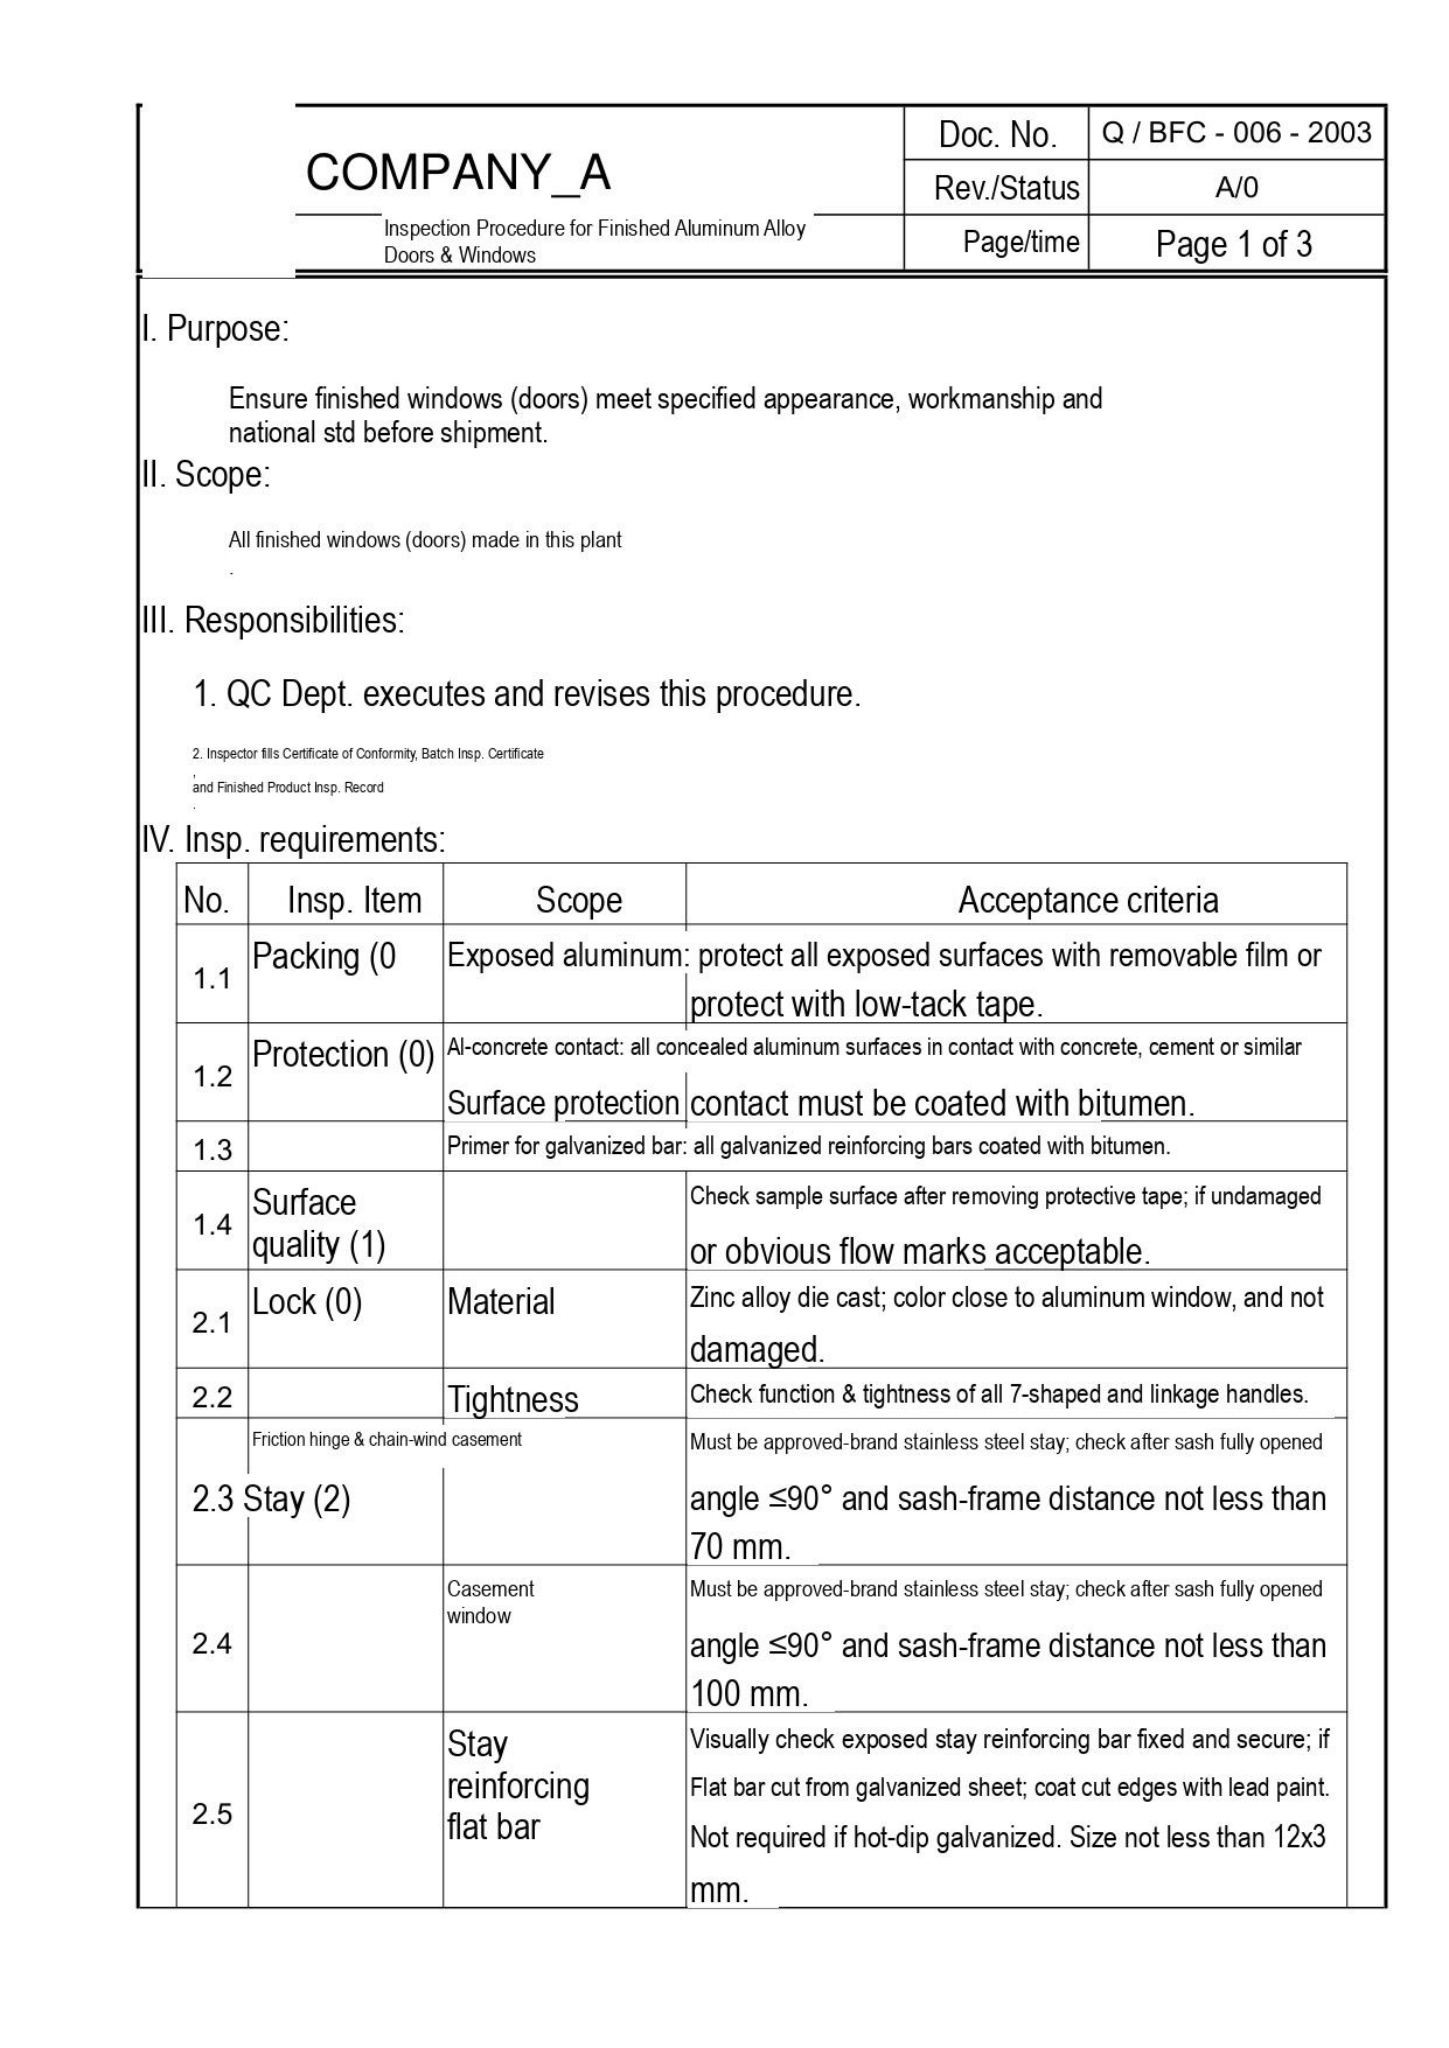COMPANY_A

Inspection Procedure for Finished Aluminum Alloy Doors & Windows

| Doc. No. | Q / BFC - 006 - 2003 |
|---|---|
| Rev./Status | A/0 |
| Page/time | Page 1 of 3 |

I. Purpose:

Ensure finished windows (doors) meet specified appearance, workmanship and national std before shipment.

II. Scope:

All finished windows (doors) made in this plant

III. Responsibilities:

1. QC Dept. executes and revises this procedure.

2. Inspector fills Certificate of Conformity, Batch Insp. Certificate and Finished Product Insp. Record

IV. Insp. requirements:

| No. | Insp. Item | Scope | Acceptance criteria |
|---|---|---|---|
| 1.1 | Packing (0 | Exposed aluminum: | protect all exposed surfaces with removable film or protect with low-tack tape. |
| 1.2 | Protection (0) | Al-concrete contact: Surface protection | all concealed aluminum surfaces in contact with concrete, cement or similar contact must be coated with bitumen. |
| 1.3 | | Primer for galvanized bar: | all galvanized reinforcing bars coated with bitumen. |
| 1.4 | Surface quality (1) | | Check sample surface after removing protective tape; if undamaged or obvious flow marks acceptable. |
| 2.1 | Lock (0) | Material | Zinc alloy die cast; color close to aluminum window, and not damaged. |
| 2.2 | | Tightness | Check function & tightness of all 7-shaped and linkage handles. |
| 2.3 | Stay (2) | Friction hinge & chain-wind casement | Must be approved-brand stainless steel stay; check after sash fully opened angle ≤90° and sash-frame distance not less than 70 mm. |
| 2.4 | | Casement window | Must be approved-brand stainless steel stay; check after sash fully opened angle ≤90° and sash-frame distance not less than 100 mm. |
| 2.5 | | Stay reinforcing flat bar | Visually check exposed stay reinforcing bar fixed and secure; if Flat bar cut from galvanized sheet; coat cut edges with lead paint. Not required if hot-dip galvanized. Size not less than 12x3 mm. |
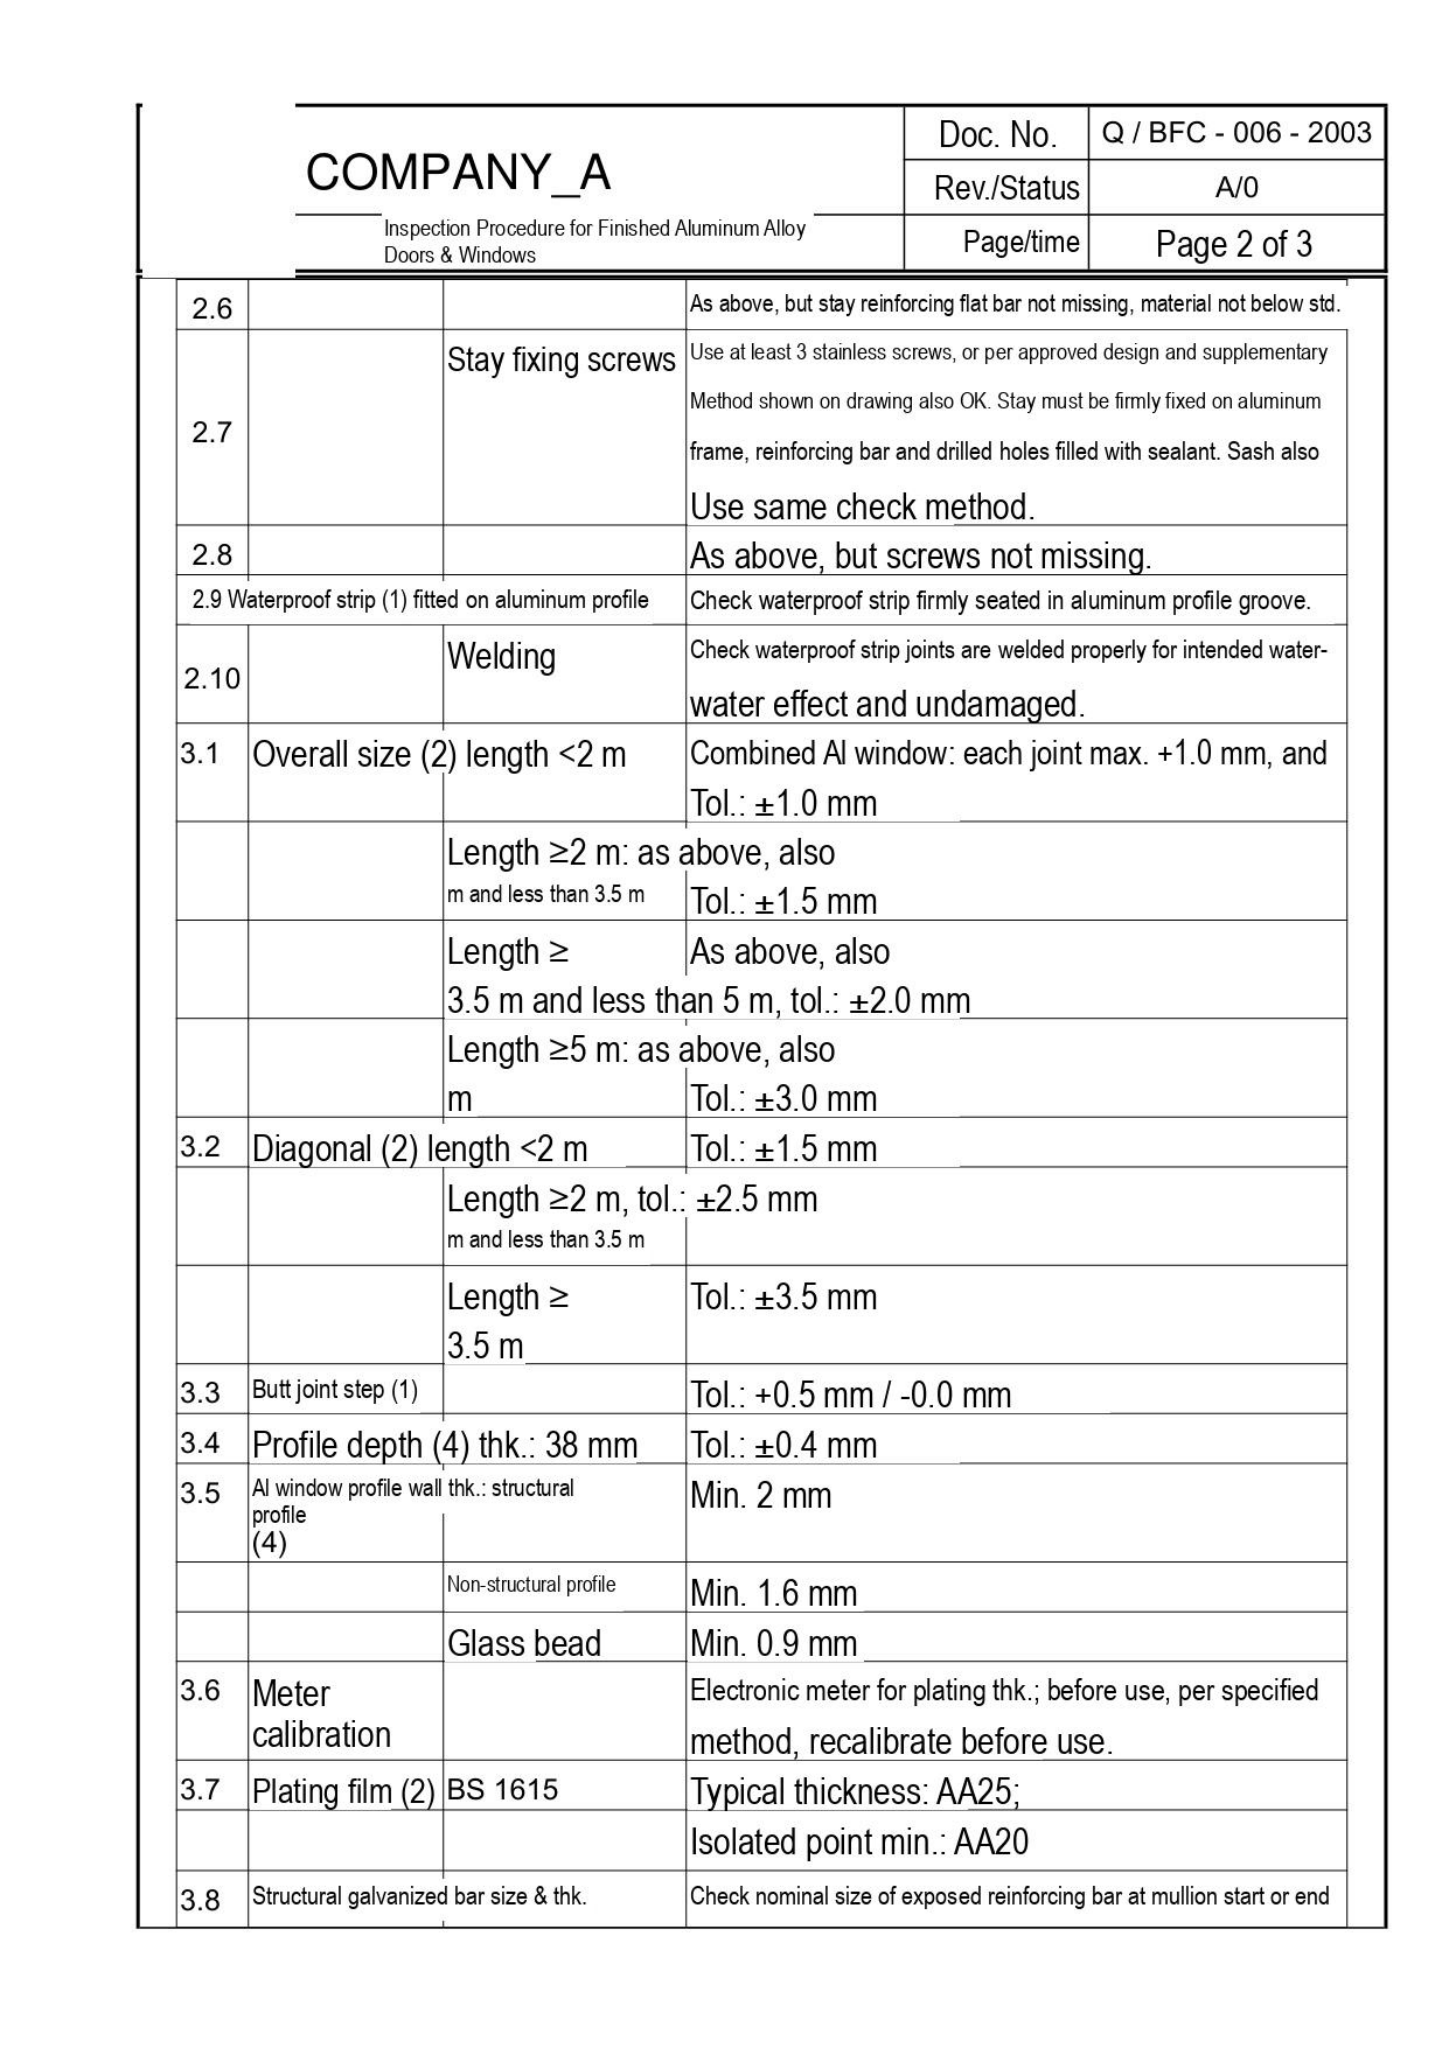| COMPANY_A<br>Inspection Procedure for Finished Aluminum Alloy Doors & Windows | Doc. No. | Q / BFC - 006 - 2003 |
|---|---|---|
| | Rev./Status | A/0 |
| | Page/time | Page 2 of 3 |

| | | | |
|---|---|---|---|
| 2.6 | | | As above, but stay reinforcing flat bar not missing, material not below std. |
| 2.7 | | Stay fixing screws | Use at least 3 stainless screws, or per approved design and supplementary Method shown on drawing also OK. Stay must be firmly fixed on aluminum frame, reinforcing bar and drilled holes filled with sealant. Sash also Use same check method. |
| 2.8 | | | As above, but screws not missing. |
| 2.9 Waterproof strip (1) fitted on aluminum profile | | | Check waterproof strip firmly seated in aluminum profile groove. |
| 2.10 | | Welding | Check waterproof strip joints are welded properly for intended water-water effect and undamaged. |
| 3.1 | Overall size (2) length <2 m | | Combined Al window: each joint max. +1.0 mm, and Tol.: ±1.0 mm |
| | | Length ≥2 m: as above, also m and less than 3.5 m | Tol.: ±1.5 mm |
| | | Length ≥ 3.5 m and less than 5 m, tol.: ±2.0 mm | As above, also |
| | | Length ≥5 m: as above, also m | Tol.: ±3.0 mm |
| 3.2 | Diagonal (2) length <2 m | | Tol.: ±1.5 mm |
| | | Length ≥2 m, tol.: ±2.5 mm m and less than 3.5 m | |
| | | Length ≥ 3.5 m | Tol.: ±3.5 mm |
| 3.3 | Butt joint step (1) | | Tol.: +0.5 mm / -0.0 mm |
| 3.4 | Profile depth (4) thk.: 38 mm | | Tol.: ±0.4 mm |
| 3.5 | Al window profile wall thk.: structural profile (4) | | Min. 2 mm |
| | | Non-structural profile | Min. 1.6 mm |
| | | Glass bead | Min. 0.9 mm |
| 3.6 | Meter calibration | | Electronic meter for plating thk.; before use, per specified method, recalibrate before use. |
| 3.7 | Plating film (2) | BS 1615 | Typical thickness: AA25; |
| | | | Isolated point min.: AA20 |
| 3.8 | Structural galvanized bar size & thk. | | Check nominal size of exposed reinforcing bar at mullion start or end |
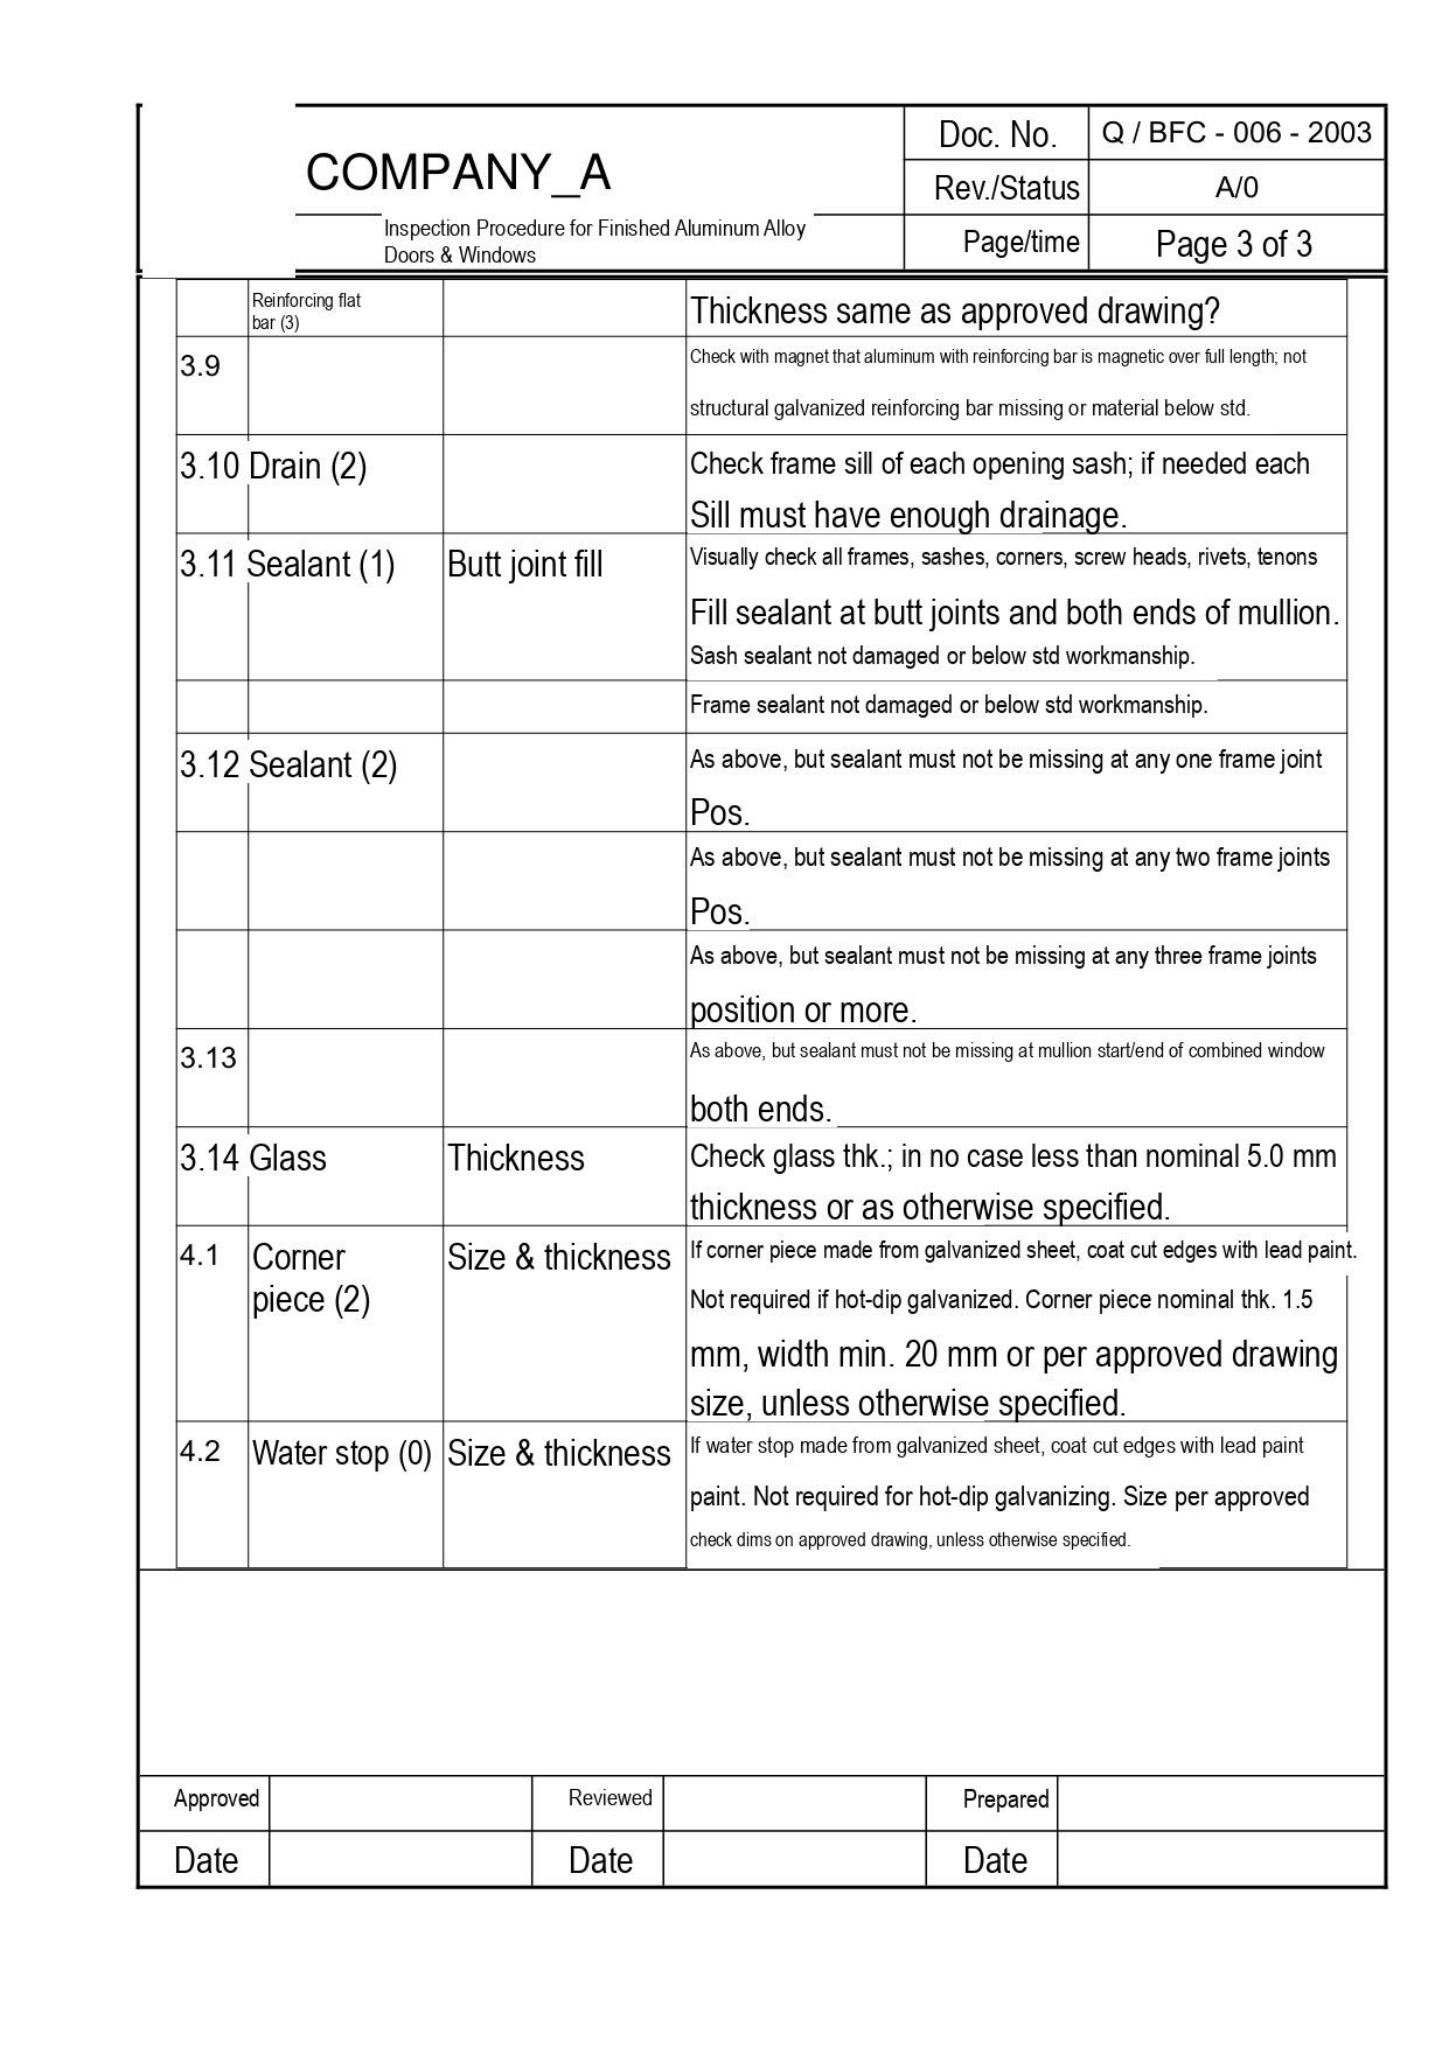COMPANY_A

Inspection Procedure for Finished Aluminum Alloy Doors & Windows

| Doc. No. | Q / BFC - 006 - 2003 |
|---|---|
| Rev./Status | A/0 |
| Page/time | Page 3 of 3 |

| | | | |
|---|---|---|---|
| | Reinforcing flat bar (3) | | Thickness same as approved drawing? |
| 3.9 | | | Check with magnet that aluminum with reinforcing bar is magnetic over full length; not structural galvanized reinforcing bar missing or material below std. |
| 3.10 | Drain (2) | | Check frame sill of each opening sash; if needed each Sill must have enough drainage. |
| 3.11 | Sealant (1) | Butt joint fill | Visually check all frames, sashes, corners, screw heads, rivets, tenons Fill sealant at butt joints and both ends of mullion. Sash sealant not damaged or below std workmanship. |
| | | | Frame sealant not damaged or below std workmanship. |
| 3.12 | Sealant (2) | | As above, but sealant must not be missing at any one frame joint Pos. |
| | | | As above, but sealant must not be missing at any two frame joints Pos. |
| | | | As above, but sealant must not be missing at any three frame joints position or more. |
| 3.13 | | | As above, but sealant must not be missing at mullion start/end of combined window both ends. |
| 3.14 | Glass | Thickness | Check glass thk.; in no case less than nominal 5.0 mm thickness or as otherwise specified. |
| 4.1 | Corner piece (2) | Size & thickness | If corner piece made from galvanized sheet, coat cut edges with lead paint. Not required if hot-dip galvanized. Corner piece nominal thk. 1.5 mm, width min. 20 mm or per approved drawing size, unless otherwise specified. |
| 4.2 | Water stop (0) | Size & thickness | If water stop made from galvanized sheet, coat cut edges with lead paint paint. Not required for hot-dip galvanizing. Size per approved check dims on approved drawing, unless otherwise specified. |

| Approved | | Reviewed | | Prepared | |
|---|---|---|---|---|---|
| Date | | Date | | Date | |